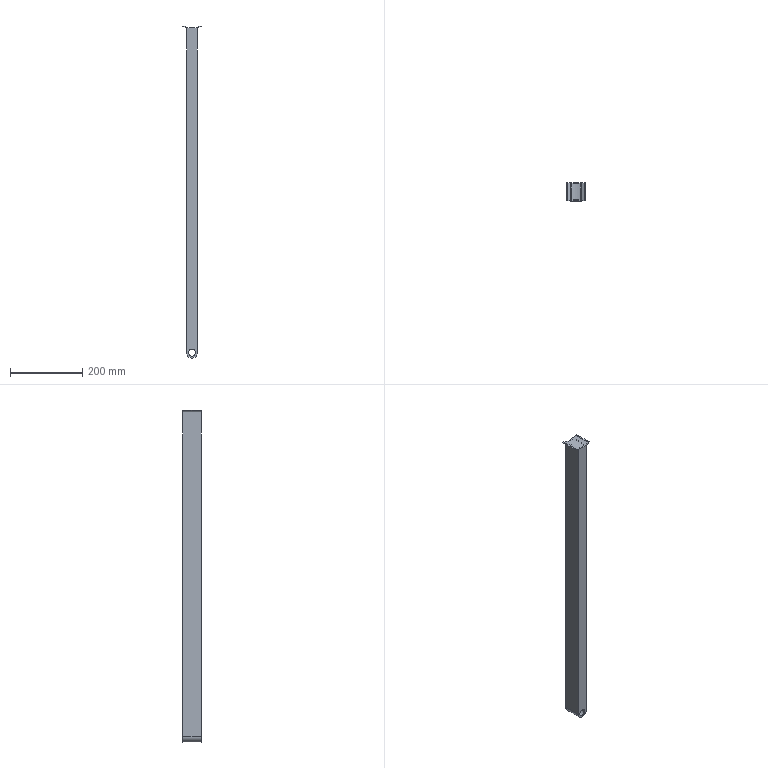Part | SolidWorks | features ICE 4, Extrusion 1 | 1 solid | 24 faces | box 54.442 x 50 x 920.099 mm | volume 408787 mm3 | plane 14 | cylinder 10 | commonest cylinder face diameters 20 x4 105.016 x3 26 x1 30 x1 101.016 x1
STEP:
#1=CARTESIAN_POINT('',(15.,0.,5.));
#2=VERTEX_POINT('',#1);
#3=CARTESIAN_POINT('',(15.,0.,25.));
#4=VERTEX_POINT('',#3);
#5=CARTESIAN_POINT('',(15.,0.,15.));
#6=DIRECTION('',(0.,1.,0.));
#7=DIRECTION('',(0.,0.,1.));
#8=AXIS2_PLACEMENT_3D('',#5,#6,#7);
#9=CIRCLE('',#8,10.);
#10=EDGE_CURVE('',#2,#4,#9,.T.);
#11=ORIENTED_EDGE('',*,*,#10,.F.);
#12=CARTESIAN_POINT('',(15.,3.,5.));
#13=VERTEX_POINT('',#12);
#14=CARTESIAN_POINT('',(15.,-850.,5.));
#15=DIRECTION('',(0.,1.,0.));
#16=VECTOR('',#15,1000.);
#17=LINE('',#14,#16);
#18=EDGE_CURVE('',#2,#13,#17,.T.);
#19=ORIENTED_EDGE('',*,*,#18,.T.);
#20=CARTESIAN_POINT('',(15.,3.,25.));
#21=VERTEX_POINT('',#20);
#22=CARTESIAN_POINT('',(15.,3.,15.));
#23=DIRECTION('',(0.,1.,0.));
#24=DIRECTION('',(0.,0.,1.));
#25=AXIS2_PLACEMENT_3D('',#22,#23,#24);
#26=CIRCLE('',#25,10.);
#27=EDGE_CURVE('',#13,#21,#26,.T.);
#28=ORIENTED_EDGE('',*,*,#27,.T.);
#29=CARTESIAN_POINT('',(15.,-850.,25.));
#30=DIRECTION('',(0.,1.,0.));
#31=VECTOR('',#30,1000.);
#32=LINE('',#29,#31);
#33=EDGE_CURVE('',#4,#21,#32,.T.);
#34=ORIENTED_EDGE('',*,*,#33,.F.);
#35=EDGE_LOOP('',(#11,#19,#28,#34));
#36=FACE_OUTER_BOUND('',#35,.T.);
#37=CARTESIAN_POINT('',(15.,-850.,15.));
#38=DIRECTION('',(0.,1.,0.));
#39=DIRECTION('',(0.,0.,1.));
#40=AXIS2_PLACEMENT_3D('',#37,#38,#39);
#41=CYLINDRICAL_SURFACE('',#40,10.);
#42=ADVANCED_FACE('',(#36),#41,.F.);
#43=CARTESIAN_POINT('',(15.,47.,25.));
#44=VERTEX_POINT('',#43);
#45=CARTESIAN_POINT('',(15.,47.,5.));
#46=VERTEX_POINT('',#45);
#47=CARTESIAN_POINT('',(15.,47.,15.));
#48=DIRECTION('',(0.,-1.,0.));
#49=DIRECTION('',(0.,0.,-1.));
#50=AXIS2_PLACEMENT_3D('',#47,#48,#49);
#51=CIRCLE('',#50,10.);
#52=EDGE_CURVE('',#44,#46,#51,.T.);
#53=ORIENTED_EDGE('',*,*,#52,.T.);
#54=CARTESIAN_POINT('',(15.,50.,5.));
#55=VERTEX_POINT('',#54);
#56=CARTESIAN_POINT('',(15.,-850.,5.));
#57=DIRECTION('',(0.,1.,0.));
#58=VECTOR('',#57,1000.);
#59=LINE('',#56,#58);
#60=EDGE_CURVE('',#46,#55,#59,.T.);
#61=ORIENTED_EDGE('',*,*,#60,.T.);
#62=CARTESIAN_POINT('',(15.,50.,25.));
#63=VERTEX_POINT('',#62);
#64=CARTESIAN_POINT('',(15.,50.,15.));
#65=DIRECTION('',(0.,1.,0.));
#66=DIRECTION('',(0.,0.,1.));
#67=AXIS2_PLACEMENT_3D('',#64,#65,#66);
#68=CIRCLE('',#67,10.);
#69=EDGE_CURVE('',#55,#63,#68,.T.);
#70=ORIENTED_EDGE('',*,*,#69,.T.);
#71=CARTESIAN_POINT('',(15.,-850.,25.));
#72=DIRECTION('',(0.,1.,0.));
#73=VECTOR('',#72,1000.);
#74=LINE('',#71,#73);
#75=EDGE_CURVE('',#44,#63,#74,.T.);
#76=ORIENTED_EDGE('',*,*,#75,.F.);
#77=EDGE_LOOP('',(#53,#61,#70,#76));
#78=FACE_OUTER_BOUND('',#77,.T.);
#79=CARTESIAN_POINT('',(15.,-850.,15.));
#80=DIRECTION('',(0.,1.,0.));
#81=DIRECTION('',(0.,0.,1.));
#82=AXIS2_PLACEMENT_3D('',#79,#80,#81);
#83=CYLINDRICAL_SURFACE('',#82,10.);
#84=ADVANCED_FACE('',(#78),#83,.F.);
#85=CARTESIAN_POINT('',(7.854,3.,915.));
#86=VERTEX_POINT('',#85);
#87=CARTESIAN_POINT('',(22.146,3.,915.));
#88=VERTEX_POINT('',#87);
#89=CARTESIAN_POINT('',(15.,3.,965.));
#90=DIRECTION('',(0.,-1.,0.));
#91=DIRECTION('',(0.,0.,1.));
#92=AXIS2_PLACEMENT_3D('',#89,#90,#91);
#93=CIRCLE('',#92,50.508);
#94=EDGE_CURVE('',#86,#88,#93,.T.);
#95=ORIENTED_EDGE('',*,*,#94,.F.);
#96=CARTESIAN_POINT('',(3.,3.,915.));
#97=DIRECTION('',(1.,0.,0.));
#98=VECTOR('',#97,1000.);
#99=LINE('',#96,#98);
#100=EDGE_CURVE('',#86,#88,#99,.T.);
#101=ORIENTED_EDGE('',*,*,#100,.T.);
#102=EDGE_LOOP('',(#95,#101));
#103=FACE_OUTER_BOUND('',#102,.T.);
#104=CARTESIAN_POINT('',(27.,3.,900.));
#105=DIRECTION('',(0.,1.,0.));
#106=DIRECTION('',(0.,0.,1.));
#107=AXIS2_PLACEMENT_3D('',#104,#105,#106);
#108=PLANE('',#107);
#109=ADVANCED_FACE('',(#103),#108,.T.);
#110=CARTESIAN_POINT('',(22.146,47.,915.));
#111=VERTEX_POINT('',#110);
#112=CARTESIAN_POINT('',(7.854,47.,915.));
#113=VERTEX_POINT('',#112);
#114=CARTESIAN_POINT('',(15.,47.,965.));
#115=DIRECTION('',(0.,1.,0.));
#116=DIRECTION('',(0.,0.,-1.));
#117=AXIS2_PLACEMENT_3D('',#114,#115,#116);
#118=CIRCLE('',#117,50.508);
#119=EDGE_CURVE('',#111,#113,#118,.T.);
#120=ORIENTED_EDGE('',*,*,#119,.F.);
#121=CARTESIAN_POINT('',(27.,47.,915.));
#122=DIRECTION('',(-1.,0.,0.));
#123=VECTOR('',#122,1000.);
#124=LINE('',#121,#123);
#125=EDGE_CURVE('',#111,#113,#124,.T.);
#126=ORIENTED_EDGE('',*,*,#125,.T.);
#127=EDGE_LOOP('',(#120,#126));
#128=FACE_OUTER_BOUND('',#127,.T.);
#129=CARTESIAN_POINT('',(3.,47.,900.));
#130=DIRECTION('',(0.,-1.,0.));
#131=DIRECTION('',(0.,0.,-1.));
#132=AXIS2_PLACEMENT_3D('',#129,#130,#131);
#133=PLANE('',#132);
#134=ADVANCED_FACE('',(#128),#133,.T.);
#135=CARTESIAN_POINT('',(22.146,50.,915.));
#136=VERTEX_POINT('',#135);
#137=CARTESIAN_POINT('',(22.146,0.,915.));
#138=DIRECTION('',(0.,-1.,0.));
#139=VECTOR('',#138,1000.);
#140=LINE('',#137,#139);
#141=EDGE_CURVE('',#136,#111,#140,.T.);
#142=ORIENTED_EDGE('',*,*,#141,.F.);
#143=CARTESIAN_POINT('',(7.854,50.,915.));
#144=VERTEX_POINT('',#143);
#145=CARTESIAN_POINT('',(30.,50.,915.));
#146=DIRECTION('',(-1.,0.,0.));
#147=VECTOR('',#146,1000.);
#148=LINE('',#145,#147);
#149=EDGE_CURVE('',#136,#144,#148,.T.);
#150=ORIENTED_EDGE('',*,*,#149,.T.);
#151=CARTESIAN_POINT('',(7.854,0.,915.));
#152=DIRECTION('',(0.,1.,0.));
#153=VECTOR('',#152,1000.);
#154=LINE('',#151,#153);
#155=EDGE_CURVE('',#113,#144,#154,.T.);
#156=ORIENTED_EDGE('',*,*,#155,.F.);
#157=ORIENTED_EDGE('',*,*,#125,.F.);
#158=EDGE_LOOP('',(#142,#150,#156,#157));
#159=FACE_OUTER_BOUND('',#158,.T.);
#160=CARTESIAN_POINT('',(0.,0.,915.));
#161=DIRECTION('',(0.,0.,1.));
#162=DIRECTION('',(1.,0.,0.));
#163=AXIS2_PLACEMENT_3D('',#160,#161,#162);
#164=PLANE('',#163);
#165=ADVANCED_FACE('',(#159),#164,.T.);
#166=CARTESIAN_POINT('',(30.,0.,914.68));
#167=VERTEX_POINT('',#166);
#168=CARTESIAN_POINT('',(30.,0.,15.));
#169=VERTEX_POINT('',#168);
#170=CARTESIAN_POINT('',(30.,0.,900.));
#171=DIRECTION('',(0.,0.,-1.));
#172=VECTOR('',#171,1000.);
#173=LINE('',#170,#172);
#174=EDGE_CURVE('',#167,#169,#173,.T.);
#175=ORIENTED_EDGE('',*,*,#174,.F.);
#176=CARTESIAN_POINT('',(42.221,0.,920.099));
#177=VERTEX_POINT('',#176);
#178=CARTESIAN_POINT('',(15.,0.,965.));
#179=DIRECTION('',(0.,1.,0.));
#180=DIRECTION('',(0.,0.,1.));
#181=AXIS2_PLACEMENT_3D('',#178,#179,#180);
#182=CIRCLE('',#181,52.508);
#183=EDGE_CURVE('',#177,#167,#182,.T.);
#184=ORIENTED_EDGE('',*,*,#183,.F.);
#185=CARTESIAN_POINT('',(38.129,0.,920.099));
#186=VERTEX_POINT('',#185);
#187=CARTESIAN_POINT('',(38.129,0.,920.099));
#188=DIRECTION('',(1.,0.,0.));
#189=VECTOR('',#188,1000.);
#190=LINE('',#187,#189);
#191=EDGE_CURVE('',#186,#177,#190,.T.);
#192=ORIENTED_EDGE('',*,*,#191,.F.);
#193=CARTESIAN_POINT('',(22.146,0.,915.));
#194=VERTEX_POINT('',#193);
#195=CARTESIAN_POINT('',(15.,0.,965.));
#196=DIRECTION('',(0.,-1.,0.));
#197=DIRECTION('',(0.,0.,1.));
#198=AXIS2_PLACEMENT_3D('',#195,#196,#197);
#199=CIRCLE('',#198,50.508);
#200=EDGE_CURVE('',#194,#186,#199,.T.);
#201=ORIENTED_EDGE('',*,*,#200,.F.);
#202=CARTESIAN_POINT('',(7.854,0.,915.));
#203=VERTEX_POINT('',#202);
#204=CARTESIAN_POINT('',(0.,0.,915.));
#205=DIRECTION('',(1.,0.,0.));
#206=VECTOR('',#205,1000.);
#207=LINE('',#204,#206);
#208=EDGE_CURVE('',#203,#194,#207,.T.);
#209=ORIENTED_EDGE('',*,*,#208,.F.);
#210=CARTESIAN_POINT('',(-8.129,0.,920.099));
#211=VERTEX_POINT('',#210);
#212=CARTESIAN_POINT('',(15.,0.,965.));
#213=DIRECTION('',(0.,-1.,0.));
#214=DIRECTION('',(0.,0.,1.));
#215=AXIS2_PLACEMENT_3D('',#212,#213,#214);
#216=CIRCLE('',#215,50.508);
#217=EDGE_CURVE('',#211,#203,#216,.T.);
#218=ORIENTED_EDGE('',*,*,#217,.F.);
#219=CARTESIAN_POINT('',(-12.221,0.,920.099));
#220=VERTEX_POINT('',#219);
#221=CARTESIAN_POINT('',(-12.221,0.,920.099));
#222=DIRECTION('',(1.,0.,0.));
#223=VECTOR('',#222,1000.);
#224=LINE('',#221,#223);
#225=EDGE_CURVE('',#220,#211,#224,.T.);
#226=ORIENTED_EDGE('',*,*,#225,.F.);
#227=CARTESIAN_POINT('',(0.,0.,914.68));
#228=VERTEX_POINT('',#227);
#229=CARTESIAN_POINT('',(15.,0.,965.));
#230=DIRECTION('',(0.,1.,0.));
#231=DIRECTION('',(0.,0.,1.));
#232=AXIS2_PLACEMENT_3D('',#229,#230,#231);
#233=CIRCLE('',#232,52.508);
#234=EDGE_CURVE('',#228,#220,#233,.T.);
#235=ORIENTED_EDGE('',*,*,#234,.F.);
#236=CARTESIAN_POINT('',(0.,0.,15.));
#237=VERTEX_POINT('',#236);
#238=CARTESIAN_POINT('',(0.,0.,900.));
#239=DIRECTION('',(0.,0.,-1.));
#240=VECTOR('',#239,1000.);
#241=LINE('',#238,#240);
#242=EDGE_CURVE('',#228,#237,#241,.T.);
#243=ORIENTED_EDGE('',*,*,#242,.T.);
#244=CARTESIAN_POINT('',(15.,0.,15.));
#245=DIRECTION('',(0.,1.,0.));
#246=DIRECTION('',(0.,0.,1.));
#247=AXIS2_PLACEMENT_3D('',#244,#245,#246);
#248=CIRCLE('',#247,15.);
#249=EDGE_CURVE('',#169,#237,#248,.T.);
#250=ORIENTED_EDGE('',*,*,#249,.F.);
#251=EDGE_LOOP('',(#175,#184,#192,#201,#209,#218,#226,#235,#243,#250));
#252=FACE_OUTER_BOUND('',#251,.T.);
#253=CARTESIAN_POINT('',(15.,0.,15.));
#254=DIRECTION('',(0.,1.,0.));
#255=DIRECTION('',(0.,0.,1.));
#256=AXIS2_PLACEMENT_3D('',#253,#254,#255);
#257=CIRCLE('',#256,10.);
#258=EDGE_CURVE('',#4,#2,#257,.T.);
#259=ORIENTED_EDGE('',*,*,#258,.T.);
#260=ORIENTED_EDGE('',*,*,#10,.T.);
#261=EDGE_LOOP('',(#259,#260));
#262=FACE_BOUND('',#261,.T.);
#263=CARTESIAN_POINT('',(30.,0.,900.));
#264=DIRECTION('',(0.,1.,0.));
#265=DIRECTION('',(0.,0.,1.));
#266=AXIS2_PLACEMENT_3D('',#263,#264,#265);
#267=PLANE('',#266);
#268=ADVANCED_FACE('',(#252,#262),#267,.F.);
#269=CARTESIAN_POINT('',(15.,50.,15.));
#270=DIRECTION('',(0.,1.,0.));
#271=DIRECTION('',(0.,0.,1.));
#272=AXIS2_PLACEMENT_3D('',#269,#270,#271);
#273=CIRCLE('',#272,10.);
#274=EDGE_CURVE('',#63,#55,#273,.T.);
#275=ORIENTED_EDGE('',*,*,#274,.F.);
#276=ORIENTED_EDGE('',*,*,#69,.F.);
#277=EDGE_LOOP('',(#275,#276));
#278=FACE_BOUND('',#277,.T.);
#279=CARTESIAN_POINT('',(0.,50.,914.68));
#280=VERTEX_POINT('',#279);
#281=CARTESIAN_POINT('',(0.,50.,15.));
#282=VERTEX_POINT('',#281);
#283=CARTESIAN_POINT('',(0.,50.,900.));
#284=DIRECTION('',(0.,0.,-1.));
#285=VECTOR('',#284,1000.);
#286=LINE('',#283,#285);
#287=EDGE_CURVE('',#280,#282,#286,.T.);
#288=ORIENTED_EDGE('',*,*,#287,.F.);
#289=CARTESIAN_POINT('',(-12.221,50.,920.099));
#290=VERTEX_POINT('',#289);
#291=CARTESIAN_POINT('',(15.,50.,965.));
#292=DIRECTION('',(0.,1.,0.));
#293=DIRECTION('',(0.,0.,1.));
#294=AXIS2_PLACEMENT_3D('',#291,#292,#293);
#295=CIRCLE('',#294,52.508);
#296=EDGE_CURVE('',#280,#290,#295,.T.);
#297=ORIENTED_EDGE('',*,*,#296,.T.);
#298=CARTESIAN_POINT('',(-8.129,50.,920.099));
#299=VERTEX_POINT('',#298);
#300=CARTESIAN_POINT('',(-12.221,50.,920.099));
#301=DIRECTION('',(1.,0.,0.));
#302=VECTOR('',#301,1000.);
#303=LINE('',#300,#302);
#304=EDGE_CURVE('',#290,#299,#303,.T.);
#305=ORIENTED_EDGE('',*,*,#304,.T.);
#306=CARTESIAN_POINT('',(15.,50.,965.));
#307=DIRECTION('',(0.,-1.,0.));
#308=DIRECTION('',(0.,0.,1.));
#309=AXIS2_PLACEMENT_3D('',#306,#307,#308);
#310=CIRCLE('',#309,50.508);
#311=EDGE_CURVE('',#299,#144,#310,.T.);
#312=ORIENTED_EDGE('',*,*,#311,.T.);
#313=ORIENTED_EDGE('',*,*,#149,.F.);
#314=CARTESIAN_POINT('',(38.129,50.,920.099));
#315=VERTEX_POINT('',#314);
#316=CARTESIAN_POINT('',(15.,50.,965.));
#317=DIRECTION('',(0.,-1.,0.));
#318=DIRECTION('',(0.,0.,1.));
#319=AXIS2_PLACEMENT_3D('',#316,#317,#318);
#320=CIRCLE('',#319,50.508);
#321=EDGE_CURVE('',#136,#315,#320,.T.);
#322=ORIENTED_EDGE('',*,*,#321,.T.);
#323=CARTESIAN_POINT('',(42.221,50.,920.099));
#324=VERTEX_POINT('',#323);
#325=CARTESIAN_POINT('',(38.129,50.,920.099));
#326=DIRECTION('',(1.,0.,0.));
#327=VECTOR('',#326,1000.);
#328=LINE('',#325,#327);
#329=EDGE_CURVE('',#315,#324,#328,.T.);
#330=ORIENTED_EDGE('',*,*,#329,.T.);
#331=CARTESIAN_POINT('',(30.,50.,914.68));
#332=VERTEX_POINT('',#331);
#333=CARTESIAN_POINT('',(15.,50.,965.));
#334=DIRECTION('',(0.,1.,0.));
#335=DIRECTION('',(0.,0.,1.));
#336=AXIS2_PLACEMENT_3D('',#333,#334,#335);
#337=CIRCLE('',#336,52.508);
#338=EDGE_CURVE('',#324,#332,#337,.T.);
#339=ORIENTED_EDGE('',*,*,#338,.T.);
#340=CARTESIAN_POINT('',(30.,50.,15.));
#341=VERTEX_POINT('',#340);
#342=CARTESIAN_POINT('',(30.,50.,900.));
#343=DIRECTION('',(0.,0.,-1.));
#344=VECTOR('',#343,1000.);
#345=LINE('',#342,#344);
#346=EDGE_CURVE('',#332,#341,#345,.T.);
#347=ORIENTED_EDGE('',*,*,#346,.T.);
#348=CARTESIAN_POINT('',(15.,50.,15.));
#349=DIRECTION('',(0.,1.,0.));
#350=DIRECTION('',(0.,0.,1.));
#351=AXIS2_PLACEMENT_3D('',#348,#349,#350);
#352=CIRCLE('',#351,15.);
#353=EDGE_CURVE('',#341,#282,#352,.T.);
#354=ORIENTED_EDGE('',*,*,#353,.T.);
#355=EDGE_LOOP('',(#288,#297,#305,#312,#313,#322,#330,#339,#347,#354));
#356=FACE_OUTER_BOUND('',#355,.T.);
#357=CARTESIAN_POINT('',(0.,50.,900.));
#358=DIRECTION('',(0.,-1.,0.));
#359=DIRECTION('',(0.,0.,-1.));
#360=AXIS2_PLACEMENT_3D('',#357,#358,#359);
#361=PLANE('',#360);
#362=ADVANCED_FACE('',(#278,#356),#361,.F.);
#363=CARTESIAN_POINT('',(27.,3.,913.882));
#364=VERTEX_POINT('',#363);
#365=CARTESIAN_POINT('',(3.,3.,913.882));
#366=VERTEX_POINT('',#365);
#367=CARTESIAN_POINT('',(15.,3.,965.));
#368=DIRECTION('',(0.,1.,0.));
#369=DIRECTION('',(0.,0.,1.));
#370=AXIS2_PLACEMENT_3D('',#367,#368,#369);
#371=CIRCLE('',#370,52.508);
#372=EDGE_CURVE('',#364,#366,#371,.T.);
#373=ORIENTED_EDGE('',*,*,#372,.F.);
#374=CARTESIAN_POINT('',(27.,3.,10.));
#375=VERTEX_POINT('',#374);
#376=CARTESIAN_POINT('',(27.,3.,900.));
#377=DIRECTION('',(0.,0.,-1.));
#378=VECTOR('',#377,1000.);
#379=LINE('',#376,#378);
#380=EDGE_CURVE('',#364,#375,#379,.T.);
#381=ORIENTED_EDGE('',*,*,#380,.T.);
#382=CARTESIAN_POINT('',(3.,3.,10.));
#383=VERTEX_POINT('',#382);
#384=CARTESIAN_POINT('',(15.,3.,15.));
#385=DIRECTION('',(0.,-1.,0.));
#386=DIRECTION('',(0.,0.,1.));
#387=AXIS2_PLACEMENT_3D('',#384,#385,#386);
#388=CIRCLE('',#387,13.);
#389=EDGE_CURVE('',#383,#375,#388,.T.);
#390=ORIENTED_EDGE('',*,*,#389,.F.);
#391=CARTESIAN_POINT('',(3.,3.,900.));
#392=DIRECTION('',(0.,0.,-1.));
#393=VECTOR('',#392,1000.);
#394=LINE('',#391,#393);
#395=EDGE_CURVE('',#366,#383,#394,.T.);
#396=ORIENTED_EDGE('',*,*,#395,.F.);
#397=EDGE_LOOP('',(#373,#381,#390,#396));
#398=FACE_OUTER_BOUND('',#397,.T.);
#399=CARTESIAN_POINT('',(15.,3.,15.));
#400=DIRECTION('',(0.,1.,0.));
#401=DIRECTION('',(0.,0.,1.));
#402=AXIS2_PLACEMENT_3D('',#399,#400,#401);
#403=CIRCLE('',#402,10.);
#404=EDGE_CURVE('',#21,#13,#403,.T.);
#405=ORIENTED_EDGE('',*,*,#404,.F.);
#406=ORIENTED_EDGE('',*,*,#27,.F.);
#407=EDGE_LOOP('',(#405,#406));
#408=FACE_BOUND('',#407,.T.);
#409=CARTESIAN_POINT('',(27.,3.,900.));
#410=DIRECTION('',(0.,1.,0.));
#411=DIRECTION('',(0.,0.,1.));
#412=AXIS2_PLACEMENT_3D('',#409,#410,#411);
#413=PLANE('',#412);
#414=ADVANCED_FACE('',(#398,#408),#413,.T.);
#415=CARTESIAN_POINT('',(3.,47.,913.882));
#416=VERTEX_POINT('',#415);
#417=CARTESIAN_POINT('',(27.,47.,913.882));
#418=VERTEX_POINT('',#417);
#419=CARTESIAN_POINT('',(15.,47.,965.));
#420=DIRECTION('',(0.,-1.,0.));
#421=DIRECTION('',(0.,0.,-1.));
#422=AXIS2_PLACEMENT_3D('',#419,#420,#421);
#423=CIRCLE('',#422,52.508);
#424=EDGE_CURVE('',#416,#418,#423,.T.);
#425=ORIENTED_EDGE('',*,*,#424,.F.);
#426=CARTESIAN_POINT('',(3.,47.,10.));
#427=VERTEX_POINT('',#426);
#428=CARTESIAN_POINT('',(3.,47.,900.));
#429=DIRECTION('',(0.,0.,-1.));
#430=VECTOR('',#429,1000.);
#431=LINE('',#428,#430);
#432=EDGE_CURVE('',#416,#427,#431,.T.);
#433=ORIENTED_EDGE('',*,*,#432,.T.);
#434=CARTESIAN_POINT('',(27.,47.,10.));
#435=VERTEX_POINT('',#434);
#436=CARTESIAN_POINT('',(15.,47.,15.));
#437=DIRECTION('',(0.,1.,0.));
#438=DIRECTION('',(0.,0.,-1.));
#439=AXIS2_PLACEMENT_3D('',#436,#437,#438);
#440=CIRCLE('',#439,13.);
#441=EDGE_CURVE('',#435,#427,#440,.T.);
#442=ORIENTED_EDGE('',*,*,#441,.F.);
#443=CARTESIAN_POINT('',(27.,47.,900.));
#444=DIRECTION('',(0.,0.,-1.));
#445=VECTOR('',#444,1000.);
#446=LINE('',#443,#445);
#447=EDGE_CURVE('',#418,#435,#446,.T.);
#448=ORIENTED_EDGE('',*,*,#447,.F.);
#449=EDGE_LOOP('',(#425,#433,#442,#448));
#450=FACE_OUTER_BOUND('',#449,.T.);
#451=ORIENTED_EDGE('',*,*,#52,.F.);
#452=CARTESIAN_POINT('',(15.,47.,15.));
#453=DIRECTION('',(0.,-1.,0.));
#454=DIRECTION('',(0.,0.,-1.));
#455=AXIS2_PLACEMENT_3D('',#452,#453,#454);
#456=CIRCLE('',#455,10.);
#457=EDGE_CURVE('',#46,#44,#456,.T.);
#458=ORIENTED_EDGE('',*,*,#457,.F.);
#459=EDGE_LOOP('',(#451,#458));
#460=FACE_BOUND('',#459,.T.);
#461=CARTESIAN_POINT('',(3.,47.,900.));
#462=DIRECTION('',(0.,-1.,0.));
#463=DIRECTION('',(0.,0.,-1.));
#464=AXIS2_PLACEMENT_3D('',#461,#462,#463);
#465=PLANE('',#464);
#466=ADVANCED_FACE('',(#450,#460),#465,.T.);
#467=ORIENTED_EDGE('',*,*,#242,.F.);
#468=CARTESIAN_POINT('',(0.,0.,914.68));
#469=DIRECTION('',(0.,1.,0.));
#470=VECTOR('',#469,1000.);
#471=LINE('',#468,#470);
#472=EDGE_CURVE('',#228,#280,#471,.T.);
#473=ORIENTED_EDGE('',*,*,#472,.T.);
#474=ORIENTED_EDGE('',*,*,#287,.T.);
#475=CARTESIAN_POINT('',(0.,-850.,15.));
#476=DIRECTION('',(0.,1.,0.));
#477=VECTOR('',#476,1000.);
#478=LINE('',#475,#477);
#479=EDGE_CURVE('',#237,#282,#478,.T.);
#480=ORIENTED_EDGE('',*,*,#479,.F.);
#481=EDGE_LOOP('',(#467,#473,#474,#480));
#482=FACE_OUTER_BOUND('',#481,.T.);
#483=CARTESIAN_POINT('',(0.,0.,900.));
#484=DIRECTION('',(1.,0.,0.));
#485=DIRECTION('',(0.,0.,-1.));
#486=AXIS2_PLACEMENT_3D('',#483,#484,#485);
#487=PLANE('',#486);
#488=ADVANCED_FACE('',(#482),#487,.F.);
#489=CARTESIAN_POINT('',(3.,0.,913.882));
#490=DIRECTION('',(0.,1.,0.));
#491=VECTOR('',#490,1000.);
#492=LINE('',#489,#491);
#493=EDGE_CURVE('',#366,#416,#492,.T.);
#494=ORIENTED_EDGE('',*,*,#493,.F.);
#495=ORIENTED_EDGE('',*,*,#395,.T.);
#496=CARTESIAN_POINT('',(3.,0.,10.));
#497=DIRECTION('',(0.,-1.,0.));
#498=VECTOR('',#497,1000.);
#499=LINE('',#496,#498);
#500=EDGE_CURVE('',#427,#383,#499,.T.);
#501=ORIENTED_EDGE('',*,*,#500,.F.);
#502=ORIENTED_EDGE('',*,*,#432,.F.);
#503=EDGE_LOOP('',(#494,#495,#501,#502));
#504=FACE_OUTER_BOUND('',#503,.T.);
#505=CARTESIAN_POINT('',(3.,3.,900.));
#506=DIRECTION('',(1.,0.,0.));
#507=DIRECTION('',(0.,0.,-1.));
#508=AXIS2_PLACEMENT_3D('',#505,#506,#507);
#509=PLANE('',#508);
#510=ADVANCED_FACE('',(#504),#509,.T.);
#511=CARTESIAN_POINT('',(27.,0.,913.882));
#512=DIRECTION('',(0.,-1.,0.));
#513=VECTOR('',#512,1000.);
#514=LINE('',#511,#513);
#515=EDGE_CURVE('',#418,#364,#514,.T.);
#516=ORIENTED_EDGE('',*,*,#515,.F.);
#517=ORIENTED_EDGE('',*,*,#447,.T.);
#518=CARTESIAN_POINT('',(27.,0.,10.));
#519=DIRECTION('',(0.,1.,0.));
#520=VECTOR('',#519,1000.);
#521=LINE('',#518,#520);
#522=EDGE_CURVE('',#375,#435,#521,.T.);
#523=ORIENTED_EDGE('',*,*,#522,.F.);
#524=ORIENTED_EDGE('',*,*,#380,.F.);
#525=EDGE_LOOP('',(#516,#517,#523,#524));
#526=FACE_OUTER_BOUND('',#525,.T.);
#527=CARTESIAN_POINT('',(27.,47.,900.));
#528=DIRECTION('',(-1.,0.,0.));
#529=DIRECTION('',(0.,0.,1.));
#530=AXIS2_PLACEMENT_3D('',#527,#528,#529);
#531=PLANE('',#530);
#532=ADVANCED_FACE('',(#526),#531,.T.);
#533=ORIENTED_EDGE('',*,*,#346,.F.);
#534=CARTESIAN_POINT('',(30.,0.,914.68));
#535=DIRECTION('',(0.,-1.,0.));
#536=VECTOR('',#535,1000.);
#537=LINE('',#534,#536);
#538=EDGE_CURVE('',#332,#167,#537,.T.);
#539=ORIENTED_EDGE('',*,*,#538,.T.);
#540=ORIENTED_EDGE('',*,*,#174,.T.);
#541=CARTESIAN_POINT('',(30.,-850.,15.));
#542=DIRECTION('',(0.,1.,0.));
#543=VECTOR('',#542,1000.);
#544=LINE('',#541,#543);
#545=EDGE_CURVE('',#169,#341,#544,.T.);
#546=ORIENTED_EDGE('',*,*,#545,.T.);
#547=EDGE_LOOP('',(#533,#539,#540,#546));
#548=FACE_OUTER_BOUND('',#547,.T.);
#549=CARTESIAN_POINT('',(30.,50.,900.));
#550=DIRECTION('',(-1.,0.,0.));
#551=DIRECTION('',(0.,0.,1.));
#552=AXIS2_PLACEMENT_3D('',#549,#550,#551);
#553=PLANE('',#552);
#554=ADVANCED_FACE('',(#548),#553,.F.);
#555=ORIENTED_EDGE('',*,*,#479,.T.);
#556=ORIENTED_EDGE('',*,*,#353,.F.);
#557=ORIENTED_EDGE('',*,*,#545,.F.);
#558=ORIENTED_EDGE('',*,*,#249,.T.);
#559=EDGE_LOOP('',(#555,#556,#557,#558));
#560=FACE_OUTER_BOUND('',#559,.T.);
#561=CARTESIAN_POINT('',(15.,-850.,15.));
#562=DIRECTION('',(0.,1.,0.));
#563=DIRECTION('',(0.,0.,1.));
#564=AXIS2_PLACEMENT_3D('',#561,#562,#563);
#565=CYLINDRICAL_SURFACE('',#564,15.);
#566=ADVANCED_FACE('',(#560),#565,.T.);
#567=ORIENTED_EDGE('',*,*,#60,.F.);
#568=ORIENTED_EDGE('',*,*,#457,.T.);
#569=ORIENTED_EDGE('',*,*,#75,.T.);
#570=ORIENTED_EDGE('',*,*,#274,.T.);
#571=EDGE_LOOP('',(#567,#568,#569,#570));
#572=FACE_OUTER_BOUND('',#571,.T.);
#573=CARTESIAN_POINT('',(15.,-850.,15.));
#574=DIRECTION('',(0.,1.,0.));
#575=DIRECTION('',(0.,0.,1.));
#576=AXIS2_PLACEMENT_3D('',#573,#574,#575);
#577=CYLINDRICAL_SURFACE('',#576,10.);
#578=ADVANCED_FACE('',(#572),#577,.F.);
#579=ORIENTED_EDGE('',*,*,#18,.F.);
#580=ORIENTED_EDGE('',*,*,#258,.F.);
#581=ORIENTED_EDGE('',*,*,#33,.T.);
#582=ORIENTED_EDGE('',*,*,#404,.T.);
#583=EDGE_LOOP('',(#579,#580,#581,#582));
#584=FACE_OUTER_BOUND('',#583,.T.);
#585=CARTESIAN_POINT('',(15.,-850.,15.));
#586=DIRECTION('',(0.,1.,0.));
#587=DIRECTION('',(0.,0.,1.));
#588=AXIS2_PLACEMENT_3D('',#585,#586,#587);
#589=CYLINDRICAL_SURFACE('',#588,10.);
#590=ADVANCED_FACE('',(#584),#589,.F.);
#591=ORIENTED_EDGE('',*,*,#441,.T.);
#592=ORIENTED_EDGE('',*,*,#500,.T.);
#593=ORIENTED_EDGE('',*,*,#389,.T.);
#594=ORIENTED_EDGE('',*,*,#522,.T.);
#595=EDGE_LOOP('',(#591,#592,#593,#594));
#596=FACE_OUTER_BOUND('',#595,.T.);
#597=CARTESIAN_POINT('',(15.,0.,15.));
#598=DIRECTION('',(0.,1.,0.));
#599=DIRECTION('',(0.,0.,1.));
#600=AXIS2_PLACEMENT_3D('',#597,#598,#599);
#601=CYLINDRICAL_SURFACE('',#600,13.);
#602=ADVANCED_FACE('',(#596),#601,.F.);
#603=CARTESIAN_POINT('',(22.146,0.,915.));
#604=DIRECTION('',(0.,-1.,0.));
#605=VECTOR('',#604,1000.);
#606=LINE('',#603,#605);
#607=EDGE_CURVE('',#88,#194,#606,.T.);
#608=ORIENTED_EDGE('',*,*,#607,.F.);
#609=ORIENTED_EDGE('',*,*,#100,.F.);
#610=CARTESIAN_POINT('',(7.854,0.,915.));
#611=DIRECTION('',(0.,1.,0.));
#612=VECTOR('',#611,1000.);
#613=LINE('',#610,#612);
#614=EDGE_CURVE('',#203,#86,#613,.T.);
#615=ORIENTED_EDGE('',*,*,#614,.F.);
#616=ORIENTED_EDGE('',*,*,#208,.T.);
#617=EDGE_LOOP('',(#608,#609,#615,#616));
#618=FACE_OUTER_BOUND('',#617,.T.);
#619=CARTESIAN_POINT('',(0.,0.,915.));
#620=DIRECTION('',(0.,0.,1.));
#621=DIRECTION('',(1.,0.,0.));
#622=AXIS2_PLACEMENT_3D('',#619,#620,#621);
#623=PLANE('',#622);
#624=ADVANCED_FACE('',(#618),#623,.T.);
#625=ORIENTED_EDGE('',*,*,#329,.F.);
#626=CARTESIAN_POINT('',(38.129,0.,920.099));
#627=DIRECTION('',(0.,1.,0.));
#628=VECTOR('',#627,1000.);
#629=LINE('',#626,#628);
#630=EDGE_CURVE('',#186,#315,#629,.T.);
#631=ORIENTED_EDGE('',*,*,#630,.F.);
#632=ORIENTED_EDGE('',*,*,#191,.T.);
#633=CARTESIAN_POINT('',(42.221,0.,920.099));
#634=DIRECTION('',(0.,1.,0.));
#635=VECTOR('',#634,1000.);
#636=LINE('',#633,#635);
#637=EDGE_CURVE('',#177,#324,#636,.T.);
#638=ORIENTED_EDGE('',*,*,#637,.T.);
#639=EDGE_LOOP('',(#625,#631,#632,#638));
#640=FACE_OUTER_BOUND('',#639,.T.);
#641=CARTESIAN_POINT('',(38.129,0.,920.099));
#642=DIRECTION('',(0.,0.,1.));
#643=DIRECTION('',(1.,0.,0.));
#644=AXIS2_PLACEMENT_3D('',#641,#642,#643);
#645=PLANE('',#644);
#646=ADVANCED_FACE('',(#640),#645,.T.);
#647=ORIENTED_EDGE('',*,*,#304,.F.);
#648=CARTESIAN_POINT('',(-12.221,0.,920.099));
#649=DIRECTION('',(0.,1.,0.));
#650=VECTOR('',#649,1000.);
#651=LINE('',#648,#650);
#652=EDGE_CURVE('',#220,#290,#651,.T.);
#653=ORIENTED_EDGE('',*,*,#652,.F.);
#654=ORIENTED_EDGE('',*,*,#225,.T.);
#655=CARTESIAN_POINT('',(-8.129,0.,920.099));
#656=DIRECTION('',(0.,1.,0.));
#657=VECTOR('',#656,1000.);
#658=LINE('',#655,#657);
#659=EDGE_CURVE('',#211,#299,#658,.T.);
#660=ORIENTED_EDGE('',*,*,#659,.T.);
#661=EDGE_LOOP('',(#647,#653,#654,#660));
#662=FACE_OUTER_BOUND('',#661,.T.);
#663=CARTESIAN_POINT('',(-12.221,0.,920.099));
#664=DIRECTION('',(0.,0.,1.));
#665=DIRECTION('',(1.,0.,0.));
#666=AXIS2_PLACEMENT_3D('',#663,#664,#665);
#667=PLANE('',#666);
#668=ADVANCED_FACE('',(#662),#667,.T.);
#669=ORIENTED_EDGE('',*,*,#94,.T.);
#670=ORIENTED_EDGE('',*,*,#607,.T.);
#671=ORIENTED_EDGE('',*,*,#200,.T.);
#672=ORIENTED_EDGE('',*,*,#630,.T.);
#673=ORIENTED_EDGE('',*,*,#321,.F.);
#674=ORIENTED_EDGE('',*,*,#141,.T.);
#675=ORIENTED_EDGE('',*,*,#119,.T.);
#676=ORIENTED_EDGE('',*,*,#155,.T.);
#677=ORIENTED_EDGE('',*,*,#311,.F.);
#678=ORIENTED_EDGE('',*,*,#659,.F.);
#679=ORIENTED_EDGE('',*,*,#217,.T.);
#680=ORIENTED_EDGE('',*,*,#614,.T.);
#681=EDGE_LOOP('',(#669,#670,#671,#672,#673,#674,#675,#676,#677,#678,#679,#680));
#682=FACE_OUTER_BOUND('',#681,.T.);
#683=CARTESIAN_POINT('',(15.,0.,965.));
#684=DIRECTION('',(0.,1.,0.));
#685=DIRECTION('',(0.,0.,1.));
#686=AXIS2_PLACEMENT_3D('',#683,#684,#685);
#687=CYLINDRICAL_SURFACE('',#686,50.508);
#688=ADVANCED_FACE('',(#682),#687,.F.);
#689=ORIENTED_EDGE('',*,*,#538,.F.);
#690=ORIENTED_EDGE('',*,*,#338,.F.);
#691=ORIENTED_EDGE('',*,*,#637,.F.);
#692=ORIENTED_EDGE('',*,*,#183,.T.);
#693=EDGE_LOOP('',(#689,#690,#691,#692));
#694=FACE_OUTER_BOUND('',#693,.T.);
#695=CARTESIAN_POINT('',(15.,0.,965.));
#696=DIRECTION('',(0.,1.,0.));
#697=DIRECTION('',(0.,0.,1.));
#698=AXIS2_PLACEMENT_3D('',#695,#696,#697);
#699=CYLINDRICAL_SURFACE('',#698,52.508);
#700=ADVANCED_FACE('',(#694),#699,.T.);
#701=ORIENTED_EDGE('',*,*,#472,.F.);
#702=ORIENTED_EDGE('',*,*,#234,.T.);
#703=ORIENTED_EDGE('',*,*,#652,.T.);
#704=ORIENTED_EDGE('',*,*,#296,.F.);
#705=EDGE_LOOP('',(#701,#702,#703,#704));
#706=FACE_OUTER_BOUND('',#705,.T.);
#707=CARTESIAN_POINT('',(15.,0.,965.));
#708=DIRECTION('',(0.,1.,0.));
#709=DIRECTION('',(0.,0.,1.));
#710=AXIS2_PLACEMENT_3D('',#707,#708,#709);
#711=CYLINDRICAL_SURFACE('',#710,52.508);
#712=ADVANCED_FACE('',(#706),#711,.T.);
#713=ORIENTED_EDGE('',*,*,#372,.T.);
#714=ORIENTED_EDGE('',*,*,#493,.T.);
#715=ORIENTED_EDGE('',*,*,#424,.T.);
#716=ORIENTED_EDGE('',*,*,#515,.T.);
#717=EDGE_LOOP('',(#713,#714,#715,#716));
#718=FACE_OUTER_BOUND('',#717,.T.);
#719=CARTESIAN_POINT('',(15.,0.,965.));
#720=DIRECTION('',(0.,1.,0.));
#721=DIRECTION('',(0.,0.,1.));
#722=AXIS2_PLACEMENT_3D('',#719,#720,#721);
#723=CYLINDRICAL_SURFACE('',#722,52.508);
#724=ADVANCED_FACE('',(#718),#723,.T.);
#725=CLOSED_SHELL('',(#42,#84,#109,#134,#165,#268,#362,#414,#466,#488,#510,#532,#554,#566,#578,#590,#602,#624,#646,#668,#688,#700,#712,#724));
#726=MANIFOLD_SOLID_BREP('',#725);
#727=CARTESIAN_POINT('',(0.,0.,0.));
#728=DIRECTION('',(0.,0.,1.));
#729=DIRECTION('',(1.,0.,0.));
#730=AXIS2_PLACEMENT_3D('',#727,#728,#729);
#731=(LENGTH_UNIT()NAMED_UNIT(*)SI_UNIT(.MILLI.,.METRE.));
#732=UNCERTAINTY_MEASURE_WITH_UNIT(LENGTH_MEASURE(0.00001),#731,'','');
#733=(NAMED_UNIT(*)PLANE_ANGLE_UNIT()SI_UNIT($,.RADIAN.));
#734=(NAMED_UNIT(*)SI_UNIT($,.STERADIAN.)SOLID_ANGLE_UNIT());
#735=(GEOMETRIC_REPRESENTATION_CONTEXT(3)GLOBAL_UNCERTAINTY_ASSIGNED_CONTEXT((#732))GLOBAL_UNIT_ASSIGNED_CONTEXT((#731,#733,#734))REPRESENTATION_CONTEXT('',''));
#736=ADVANCED_BREP_SHAPE_REPRESENTATION('',(#726,#730),#735);